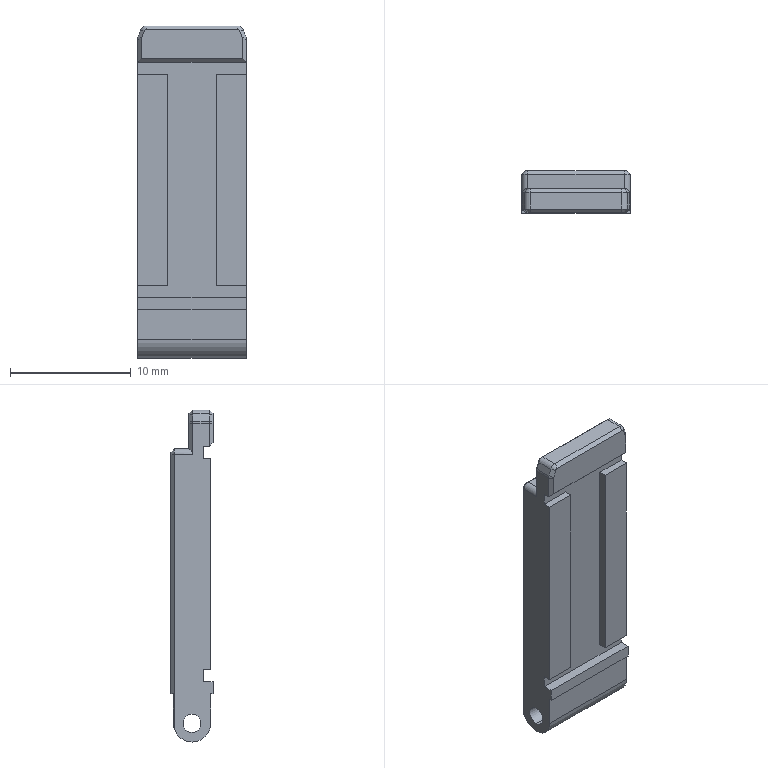Part | SolidWorks | features ICE 6, Chamfer 2, Fillet 2, Extrusion 1 | 1 solid | 59 faces | box 9 x 3.5 x 27.5 mm | volume 690.682 mm3 | plane 39 | cylinder 10 | cone 10 | commonest cylinder face diameters 1 x6 1.5 x2 3.1 x2